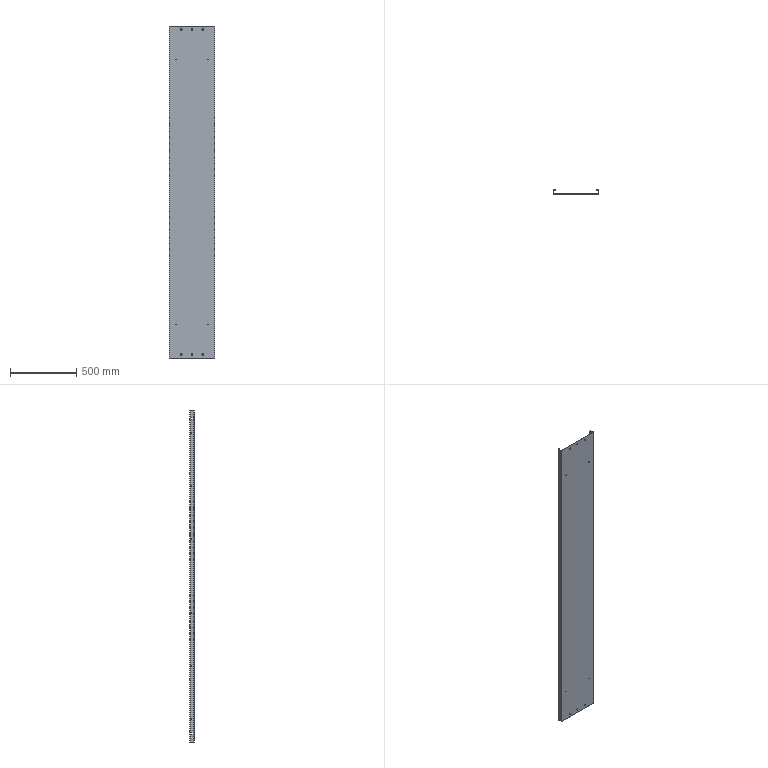Part | SolidWorks | features ICE 7, Cut 1, FlatPattern 1, SMBaseFlange 1, SheetMetal 1 | 1 solid | 122 faces | box 346 x 32 x 2502 mm | volume 1082506 mm3 | cylinder 76 | plane 46 | commonest cylinder face diameters 6.2 x48 10.5 x12 5 x8 2 x4 4 x4